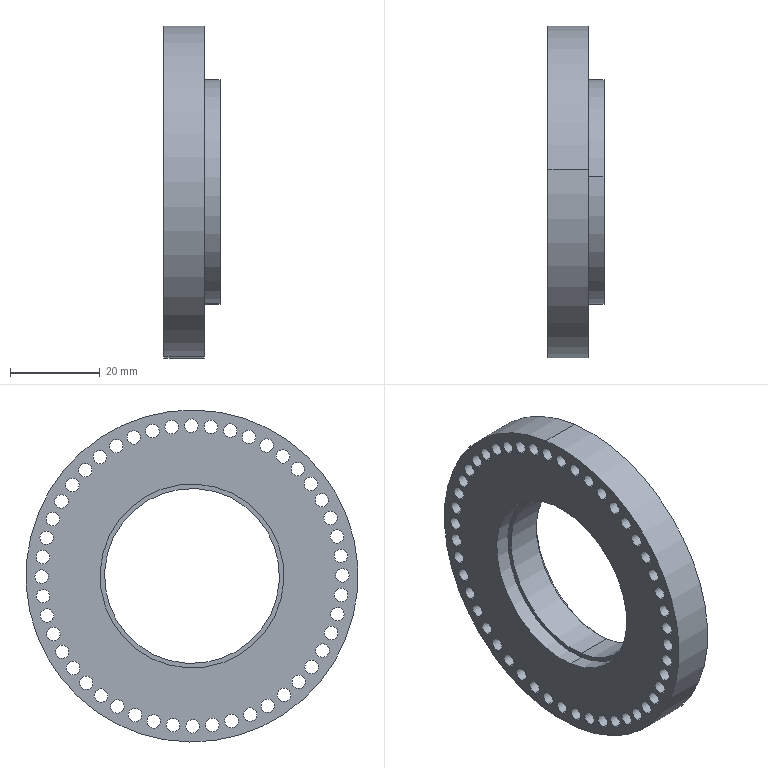Part | NX | features BREP 1 | 1 solid | 110 faces | box 12.5 x 74 x 74 mm | volume 27092 mm3 | cylinder 104 | plane 4 | cone 2 | commonest cylinder face diameters 3 x96 39 x2 41 x2 50 x2 74 x2